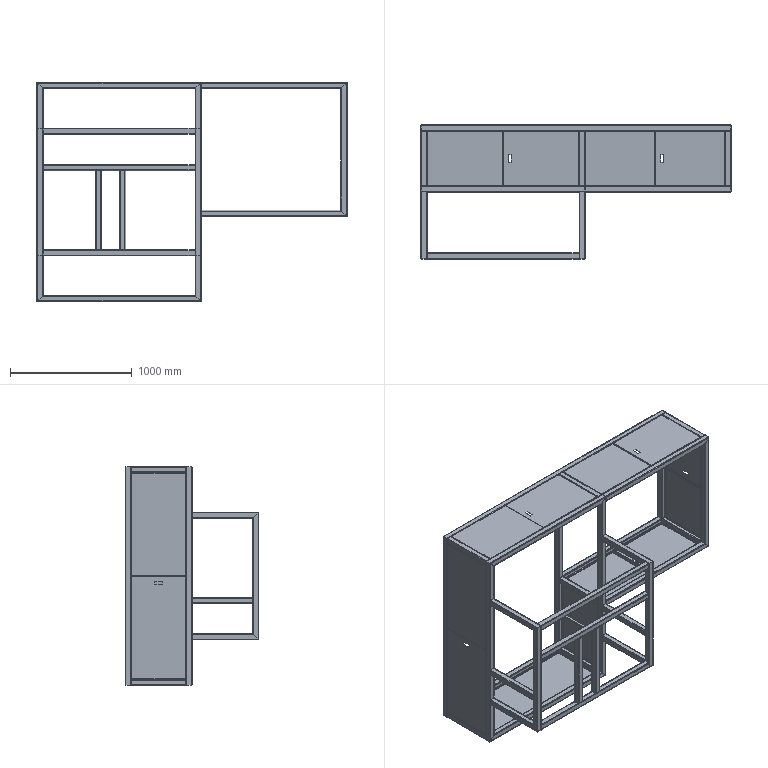Part | STEP file | 47 solids | 986 faces | box 2550 x 1100 x 1800 mm | volume 25123488 mm3 | plane 610 | cylinder 376 | commonest cylinder face diameters 6.4 x132 12.8 x132 5.2 x112